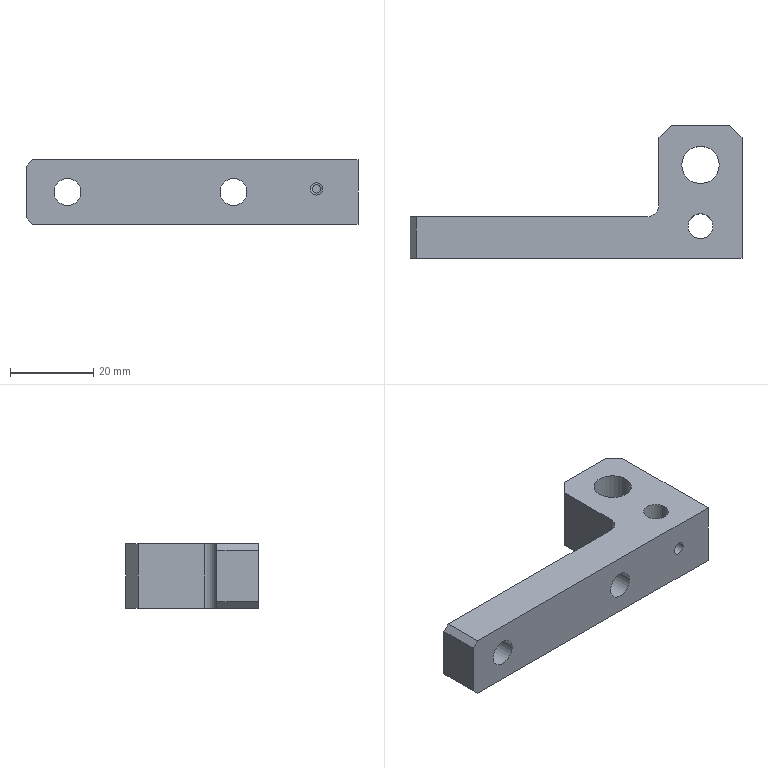NC program | NX | posted with a generic post | part box 80 x 32 x 15.5 mm
Lines 1 to 843 of 1848:
N10 G17 G21 G94 G90
(ADAPTIVE_MILLING , TOOL : D10-30-D10-75-3T-ROUGH)
N12 T01 M6
N14 G54
N16 G17 G0 G90 X-14.714 Y-27.953 B0. C0. S3000 M3
N18 G43 Z20. H1
N20 Z3.1
N22 G94 G1 X-14.735 Y-27.804 Z2.163 F1500.
N24 X-14.756 Y-27.656 Z1.792
N26 X-14.778 Y-27.507 Z1.52
N28 X-14.799 Y-27.359 Z1.3
N30 X-14.82 Y-27.21 Z1.116
N32 X-14.841 Y-27.062 Z0.958
N34 X-14.862 Y-26.913 Z0.82
N36 X-14.883 Y-26.765 Z0.7
N38 X-14.904 Y-26.616 Z0.595
N40 X-14.925 Y-26.467 Z0.502
N42 X-14.946 Y-26.319 Z0.421
N44 X-14.967 Y-26.17 Z0.35
N46 X-14.988 Y-26.022 Z0.29
N48 X-15.009 Y-25.873 Z0.238
N50 X-15.03 Y-25.725 Z0.195
N52 X-15.051 Y-25.576 Z0.161
N54 X-15.072 Y-25.428 Z0.134
N56 X-15.093 Y-25.279 Z0.115
N58 X-15.114 Y-25.131 Z0.104
N60 X-15.135 Y-24.982 Z0.1
N62 X-15.363 Y-23.368
N64 G3 X-16.363 Y-22.5 R1.01
N66 G2 X-19.774 Y-22.29 R16.737
N68 G3 X-25.917 Y-22.107 R71.98
N70 G1 X-30.851 Y-22.1
N72 G2 X-41.35 Y-22.08 R681.82
N74 X-45.596 Y-19.563 R5.775
N76 X-47.239 Y-15.194 R10.06
N78 X-47.576 Y-9.708 R40.211
N80 G1 X-47.6 Y-2.208
N82 X-47.597 Y15.46
N84 G2 X-45.145 Y20.047 R5.721
N86 X-40.851 Y21.717 R9.828
N88 X-35.168 Y22.076 R39.146
N90 G1 X-27.668 Y22.1
N92 X40.882 Y22.099
N94 G2 X45.469 Y19.73 R5.695
N96 X47.205 Y15.397 R9.72
N98 X47.575 Y9.765 R37.875
N100 G3 X47.629 Y6.228 R103.503
N102 G1 X47.728 Y5.055
N104 X47.904 Y4.474
N106 G2 X48. Y1.85 R17.179
N108 G3 X48.45 Y1.015 R1.001
N110 G1 X48.82 Y0.771
N112 X50.479 Y-0.322 Z0.2
N114 X50.822 Y-0.56 F15000.
N116 G2 X51.159 Y-1.309 R1.002
N118 G1 Y-16.392
N120 G2 X50.282 Y-20.805 R11.534
N122 G1 X49.642 Y-22.35
N124 G2 X48.185 Y-23.956 R3.345
N126 G1 X47.336 Y-24.376
N128 X46.477 Y-24.773
N130 G2 X43.308 Y-25.416 R8.24
N132 G1 X-15.817 Y-25.563
N134 G2 X-16.613 Y-25.173 R1.002
N136 G1 X-16.748 Y-24.997
N138 X-17.958 Y-23.423 Z0.1 F1500.
N140 X-18.252 Y-23.036
N142 X-18.556 Y-22.657
N144 G3 X-18.977 Y-22.403 R1.021
N146 X-22.436 Y-21.831 R12.422
N148 X-31.452 Y-21.701 R185.205
N150 G2 X-39.651 Y-21.68 R445.211
N152 X-45.227 Y-18.167 R7.162
N154 X-46.837 Y-13.315 R12.369
N156 X-47.177 Y-7.178 R49.965
N158 G1 X-47.199 Y0.522
N160 X-47.197 Y13.772
N162 G2 X-43.863 Y19.608 R7.09
N164 X-39.039 Y21.306 R11.953
N166 X-33.005 Y21.673 R45.882
N168 G1 X-25.305 Y21.699
N170 X39.193 Y21.698
N172 G2 X45.156 Y18.278 R7.123
N174 X46.818 Y13.441 R12.136
N176 X47.18 Y7.764 R49.503
N178 G3 X47.306 Y6.049 R15.738
N180 X47.62 Y5.412 R8.746
N182 G1 X47.736 Y5.029
N184 G3 X48.524 Y4.331 R1.009
N186 G1 X50.454 Y3.861 Z0.2
N188 X50.72 Y3.798 F15000.
N190 X50.983 Y3.721
N192 G2 X51.605 Y2.795 R1.001
N194 G1 Y-13.34
N196 G2 X51.071 Y-18.246 R22.814
N198 G1 X50.896 Y-19.053
N200 X50.704 Y-19.856
N202 G2 X47.108 Y-24.346 R7.33
N204 X46.142 Y-24.761 R7.288
N206 X44.228 Y-25.327 R15.44
N208 X41.944 Y-25.575 R11.567
N210 G1 X-17.413 Y-26.07
N212 G2 X-18.393 Y-25.303 R1.
N214 G1 X-18.473 Y-24.97
N216 X-18.937 Y-23.039 Z0.1 F1500.
N218 G3 X-19.508 Y-22.254 R1.059
N220 X-21.032 Y-21.765 R13.134
N222 X-25.727 Y-21.363 R28.488
N224 X-37.951 Y-21.289 R754.678
N226 G2 X-44.901 Y-16.95 R8.103
N228 X-46.45 Y-11.759 R14.331
N230 X-46.78 Y-4.971 R60.69
N232 G1 X-46.799 Y2.229
N234 X-46.783 Y12.579
N236 G2 X-42.478 Y19.387 R8.083
N238 X-37.238 Y20.954 R14.336
N240 X-30.45 Y21.28 R61.3
N242 G1 X-23.25 Y21.299
N244 X37.6 Y21.297
N246 G2 X44.907 Y16.935 R8.122
N248 X46.432 Y11.892 R14.201
N250 X46.81 Y7.334 R102.693
N252 G3 X47.059 Y6.399 R2.011
N254 X47.508 Y6.062 R1.012
N256 G1 X48.471 Y5.702
N258 X50.33 Y5.003 Z0.2
N260 G2 X50.929 Y4.165 R1.001 F15000.
N262 G1 X51.038 Y2.776
N264 X51.138 Y1.386
N266 G2 X51.198 Y-1.397 R42.642
N268 G1 X50.998 Y-17.535
N270 G2 X50.112 Y-21.491 R9.773
N272 X48.101 Y-23.985 R6.903
N274 X46.76 Y-24.887 R8.194
N276 X43.683 Y-25.648 R6.743
N278 G1 X-17.725 Y-25.965
N280 G2 X-18.686 Y-25.258 R1.
N282 G1 X-18.785 Y-24.934
N284 X-19.367 Y-23.035 Z0.1 F1500.
N286 X-19.521 Y-22.562
N288 G3 X-19.959 Y-22.095 R1.007
N290 X-22.533 Y-21.285 R6.797
N292 X-28.518 Y-20.935 R48.284
N294 G2 X-36.851 Y-20.878 R946.687
N296 X-44.518 Y-15.953 R8.819
N298 X-46.04 Y-10.591 R15.704
N300 X-46.381 Y-3.253 R67.006
N302 X-46.376 Y11.371 R824.313
N304 X-41.497 Y18.996 R8.797
N306 X-36.243 Y20.521 R15.472
N308 X-29.206 Y20.877 R62.007
N310 G1 X-22.556 Y20.898
N312 X36.044 Y20.897
N314 G2 X40.776 Y19.847 R9.724
N316 X44.932 Y15.065 R9.404
N318 X46.128 Y9.92 R18.692
N320 G3 X46.498 Y7.297 R19.933
N322 X46.7 Y6.835 R1.928
N324 G2 X47.37 Y5.88 R3.796
N326 G3 X47.958 Y5.395 R1.003
N328 G1 X48.481 Y5.234
N330 X50.379 Y4.649 Z0.2
N332 G2 X50.901 Y4.395 R1.246 F15000.
N334 X51.24 Y3.646 R1.002
N336 G1 Y-16.402
N338 G2 X50.362 Y-20.814 R11.534
N340 G1 X49.722 Y-22.36
N342 G2 X48.475 Y-23.837 R3.306
N344 G1 X48.264 Y-23.964
N346 X48.047 Y-24.08
N348 X47.306 Y-24.438
N350 X46.558 Y-24.785
N352 G2 X43.39 Y-25.434 R8.262
N354 G1 X-18.166 Y-25.729
N356 G2 X-19.127 Y-25.022 R1.
N358 G1 X-19.165 Y-24.897
N360 X-19.747 Y-22.998 Z0.1 F1500.
N362 X-19.848 Y-22.66
N364 X-19.961 Y-22.326
N366 G3 X-20.4 Y-21.859 R1.007
N368 X-23.33 Y-20.912 R7.518
N370 X-29.573 Y-20.539 R50.382
N372 G2 X-35.961 Y-20.462 R274.783
N374 X-44.066 Y-15.175 R9.369
N376 X-45.634 Y-9.52 R16.775
N378 X-45.981 Y-1.931 R71.604
N380 X-45.973 Y10.221 R586.173
N382 X-43.583 Y16.38 R9.462
N384 X-38.344 Y19.481 R11.217
N386 X-32.27 Y20.36 R26.687
N388 X-21.022 Y20.498 R255.072
N390 G1 X34.594
N392 G2 X38.925 Y19.873 R12.356
N394 X44.169 Y14.966 R9.478
N396 X45.61 Y9.987 R17.983
N398 G3 X46.186 Y7.447 R12.718
N400 G1 X46.387 Y7.162
N402 G3 X47.1 Y6.879 R1.003
N404 G1 X47.641 Y6.888
N406 X49.627 Y6.919 Z0.2
N408 G2 X50.703 Y6.005 R1.004 F15000.
N410 G1 X50.863 Y4.153
N412 X50.99 Y2.299
N414 X51.028 Y1.37
N416 X51.055 Y0.442
N418 X51.364 Y-16.831
N420 G2 X50.537 Y-20.562 R8.179
N422 G1 X50.288 Y-21.071
N424 X50.03 Y-21.576
N426 G2 X46.414 Y-24.768 R7.185
N428 X44.441 Y-25.299 R8.502
N430 X41.978 Y-25.475 R17.725
N432 G1 X-18.545 Y-25.526
N434 G2 X-19.493 Y-24.847 R1.001
N436 G1 X-20.158 Y-22.976 Z0.1 F1500.
N438 X-20.334 Y-22.47
N440 X-20.525 Y-21.97
N442 G3 X-20.779 Y-21.656 R1.063
N444 X-22.712 Y-20.797 R4.681
N446 X-27.729 Y-20.221 R26.336
N448 X-34.584 Y-20.082 R457.494
N450 G2 X-39.917 Y-18.597 R10.707
N452 X-44.138 Y-13.279 R10.563
N454 X-45.351 Y-7.32 R21.539
N456 X-45.593 Y1.724 R122.623
N458 X-45.559 Y9.373 R222.08
N460 X-43.559 Y15.194 R10.168
N462 X-38.192 Y18.849 R11.065
N464 X-32.399 Y19.884 R23.65
N466 X-23.553 Y20.093 R136.651
N468 G1 X-19.703 Y20.098
N470 X33.394 Y20.097
N472 G2 X37.65 Y19.605 R14.796
N474 X43.577 Y14.536 R9.791
N476 X45.047 Y10.239 R18.608
N478 G3 X45.719 Y7.923 R14.432
N480 X46.028 Y7.452 R1.701
N482 G2 X46.727 Y6.802 R3.41
N484 G3 X47.585 Y6.44 R1.001
N486 G1 X47.802 Y6.459
N488 X49.781 Y6.627 Z0.2
N490 G2 X50.401 Y6.58 R1.287 F15000.
N492 X51.043 Y5.646 R1.
N494 G1 Y-17.936
N496 G2 X50.402 Y-20.7 R6.428
N498 X48.791 Y-23.066 R8.698
N500 X47.097 Y-24.351 R7.72
N502 X44.507 Y-25.378 R9.704
N504 X42.88 Y-25.56 R7.773
N506 G1 X-19.777 Y-25.845
N508 G2 X-20.778 Y-24.759 R1.
N510 G1 X-20.753 Y-24.478
N512 X-20.582 Y-22.499 Z0.1 F1500.
N514 G3 X-20.934 Y-21.529 R1.045
N516 X-22.985 Y-20.51 R4.814
N518 X-27.996 Y-19.854 R24.391
N520 X-33.776 Y-19.684 R611.585
N522 G2 X-39.086 Y-18.255 R11.47
N524 X-43.596 Y-12.838 R10.785
N526 X-44.915 Y-6.75 R21.373
N528 X-45.187 Y1.644 R105.147
N530 X-45.145 Y8.593 R150.97
N532 X-43.224 Y14.396 R10.761
N534 X-37.757 Y18.316 R11.24
N536 X-31.581 Y19.47 R23.765
N538 X-22.436 Y19.693 R137.445
N540 G1 X-18.586 Y19.698
N542 X32.194 Y19.697
N544 G2 X36.561 Y19.274 R17.525
N546 X43.087 Y13.962 R10.184
N548 X44.682 Y9.777 R24.402
N550 G3 X45.475 Y7.906 R7.211
N552 G1 X45.696 Y7.705
N554 G3 X46.557 Y7.598 R1.002
N556 G1 X46.808 Y7.683
N558 X48.689 Y8.319 Z0.2
N560 G2 X49.171 Y8.436 R1.518 F15000.
N562 X50.164 Y7.705 R1.
N564 G1 X50.622 Y6.031
N566 G2 X50.941 Y4.08 R13.684
N568 G1 X51.268 Y0.429
N570 X51.578 Y-3.223
N572 G2 X51.364 Y-14.453 R62.802
N574 G1 X50.826 Y-19.388
N576 G2 X49.721 Y-22.298 R6.117
N578 X48.484 Y-23.515 R5.386
N580 G1 X47.817 Y-23.988
N582 X47.141 Y-24.451
N584 G2 X42.969 Y-25.655 R7.799
N586 G1 X-20.086 Y-25.592
N588 G2 X-21.082 Y-24.507 R1.
N590 G1 X-21.068 Y-24.343
N592 X-20.9 Y-22.364 Z0.1 F1500.
N594 G3 X-20.896 Y-21.858 R1.79
N596 X-21.243 Y-21.276 R1.006
N598 X-23.549 Y-20.135 R5.314
N600 X-28.561 Y-19.471 R25.379
N602 G2 X-33.533 Y-19.255 R236.762
N604 X-39.442 Y-17.168 R11.236
N606 X-43.388 Y-11.566 R11.676
N608 X-44.562 Y-5.242 R24.608
N610 X-44.794 Y4.904 R151.502
N612 X-44.553 Y9.391 R26.845
N614 X-38.661 Y17.215 R10.493
N616 X-32.663 Y18.872 R18.654
N618 X-24.478 Y19.274 R74.416
N620 G1 X-17.278 Y19.297
N622 X31.044 Y19.296
N624 G2 X35.617 Y18.907 R20.31
N626 X42.471 Y13.68 R10.564
N628 X44.188 Y9.842 R28.498
N630 G3 X45.156 Y8.035 R6.211
N632 X45.779 Y7.656 R2.99
N634 G1 X46.049 Y7.434
N636 G3 X47.052 Y7.277 R1.001
N638 G1 X48.847 Y8.126 Z0.2
N640 X49.037 Y8.215 F15000.
N642 X49.231 Y8.296
N644 G2 X50.518 Y7.434 R1.
N646 G1 X50.812 Y4.348
N648 X51.07 Y1.259
N650 X51.171 Y-0.287
N652 X51.257 Y-1.835
N654 X51.56 Y-8.036
N656 G2 X51.183 Y-16.678 R46.836
N658 G1 X50.845 Y-19.138
N660 G2 X47.709 Y-24.114 R7.078
N662 X46.137 Y-24.88 R7.94
N664 X42.754 Y-25.485 R9.772
N666 G1 X-19.527
N668 G2 X-20.515 Y-25.308 R3.366
N670 X-21.146 Y-24.436 R1.001
N672 G1 X-21.155 Y-24.295
N674 X-21.27 Y-22.313 Z0.1 F1500.
N676 X-21.291 Y-21.899
N678 X-21.327 Y-21.486
N680 G3 X-21.536 Y-21.034 R1.02
N682 X-23.105 Y-20.065 R3.781
N684 X-27.529 Y-19.203 R17.384
N686 X-32.711 Y-18.879 R747.688
N688 G2 X-38.324 Y-17.094 R12.112
N690 X-42.791 Y-11.371 R11.636
N692 X-44.09 Y-5.226 R22.987
N694 X-44.387 Y3.866 R110.396
N696 X-44.148 Y8.605 R29.152
N698 X-37.994 Y16.799 R10.818
N700 X-31.943 Y18.456 R19.235
N702 X-23.958 Y18.868 R72.763
N704 G1 X-15.108 Y18.897
N706 X29.992 Y18.896
N708 G2 X34.719 Y18.534 R22.942
N710 X41.806 Y13.513 R10.976
N712 X43.741 Y9.797 R34.512
N714 G3 X44.712 Y8.257 R6.177
N716 X45.37 Y7.875 R5.475
N718 X46.062 Y7.781 R1.005
N720 G1 X46.716 Y7.929
N722 X48.653 Y8.366 Z0.2
N724 G2 X49.838 Y7.875 R1.018 F15000.
N726 G1 X50.344 Y6.923
N728 X50.835 Y5.964
N730 G2 X51.491 Y2.974 R7.15
N732 G1 Y-15.114
N734 G2 X50.706 Y-19.952 R15.305
N736 G1 X50.465 Y-20.685
N738 X50.208 Y-21.413
N740 G2 X48.991 Y-23.133 R4.646
N742 X46.488 Y-24.669 R8.641
N744 X42.156 Y-25.524 R11.366
N746 G1 X-18.513 Y-25.391
N748 G2 X-20.443 Y-25.273 R19.912
N750 X-21.353 Y-24.285 R1.
N752 G1 X-21.354 Y-24.185
N754 X-21.368 Y-22.199 Z0.1 F1500.
N756 Y-21.823
N758 X-21.383 Y-21.448
N760 G3 X-21.6 Y-20.957 R1.014
N762 X-23.279 Y-19.799 R3.75
N764 X-27.648 Y-18.86 R16.456
N766 G2 X-32.453 Y-18.459 R331.016
N768 X-38.453 Y-16.169 R12.057
N770 X-42.483 Y-10.425 R12.3
N772 X-43.731 Y-3.911 R25.337
N774 X-43.908 Y6.332 R91.067
N776 X-42.178 Y12.167 R12.335
N778 X-36.453 Y16.777 R11.742
N780 X-30.074 Y18.172 R22.995
N782 X-21.182 Y18.484 R105.943
N784 G1 X-15.132 Y18.497
N786 X28.994 Y18.496
N788 G2 X33.825 Y18.162 R25.814
N790 X41.234 Y13.226 R11.502
N792 X43.295 Y9.764 R46.583
N794 G3 X44.401 Y8.324 R5.147
N796 X44.959 Y8.095 R3.127
N798 X45.997 Y8.153 R1.001
N800 G1 X46.753 Y8.795 Z0.15
N802 X47.501 Y9.448 Z0.2
N804 X47.814 Y9.706 F15000.
N806 G2 X49.275 Y9.252 R1.
N808 G1 X49.828 Y7.946
N810 X50.365 Y6.634
N812 G2 X51.08 Y2.638 R11.526
N814 G1 Y-17.377
N816 G2 X50.245 Y-20.945 R8.234
N818 X47.7 Y-24.037 R8.218
N820 X45.037 Y-25.198 R7.143
N822 X43.408 Y-25.39 R8.463
N824 X27.901 Y-25.602 R952.924
N826 G1 X-16.916 Y-25.805
N828 G2 X-19.414 Y-25.426 R8.19
N830 G1 X-20.634 Y-25.041
N832 G2 X-21.326 Y-24.204 R1.001
N834 G1 X-21.489 Y-22.224 Z0.1 F1500.
N836 X-21.567 Y-21.277
N838 G3 X-21.79 Y-20.725 R1.009
N840 X-23.62 Y-19.455 R4.102
N842 X-27.899 Y-18.503 R16.744
N844 G2 X-32.357 Y-18.012 R95.294
N846 X-38.865 Y-14.917 R11.936
N848 X-42.31 Y-9.054 R13.4
N850 X-43.39 Y-2.254 R29.777
N852 X-43.484 Y5.741 R70.346
N854 X-41.671 Y11.706 R12.569
N856 X-35.842 Y16.352 R12.01
N858 X-29.463 Y17.754 R23.409
N860 X-20.022 Y18.085 R108.737
N862 G1 X-13.422 Y18.097
N864 X27.944 Y18.096
N866 G2 X32.879 Y17.8 R29.782
N868 X40.639 Y13.003 R12.088
N870 X42.891 Y9.671 R70.619
N872 G3 X44.018 Y8.419 R4.824
N874 X44.67 Y8.193 R6.088
N876 X45.472 Y8.291 R1.002
N878 G1 X45.76 Y8.463
N880 X47.466 Y9.48 Z0.2
N882 G2 X47.945 Y9.716 R1.786 F15000.
N884 X48.986 Y9.35 R1.001
N886 G1 X49.539 Y8.603
N888 G2 X49.977 Y7.789 R5.276
N890 X50.496 Y6.446 R12.486
N892 X50.787 Y4.836 R7.473
N894 X51.502 Y-6.926 R544.363
N896 G1 X51.773 Y-12.507
N898 G2 X51.324 Y-17.403 R17.642
N900 X50.653 Y-19.783 R19.367
N902 X49.925 Y-21.486 R16.68
N904 G1 X49.596 Y-22.152
N906 X49.254 Y-22.812
N908 G2 X47.588 Y-24.203 R3.415
N910 G1 X46.8 Y-24.516
N912 X46.007 Y-24.82
N914 G2 X42.856 Y-25.409 R10.722
N916 X35.414 Y-25.572 R219.894
N918 G1 X-14.892 Y-25.77
N920 G2 X-19.629 Y-25.37 R27.069
N922 G1 X-21.98 Y-24.961
N924 G2 X-22.726 Y-23.578 R1.
N926 G1 X-22.637 Y-23.372
N928 X-21.847 Y-21.55 Z0.1 F1500.
N930 G3 X-21.98 Y-20.493 R1.002
N932 X-23.81 Y-19.167 R4.163
N934 X-28.123 Y-18.143 R16.733
N936 G2 X-32.515 Y-17.5 R48.24
N938 X-41.146 Y-10.451 R11.983
N940 X-42.773 Y-3.979 R21.871
N942 X-43.057 Y5.157 R57.101
N944 X-41.195 Y11.209 R12.776
N946 X-35.417 Y15.859 R12.175
N948 X-28.953 Y17.328 R23.307
N950 X-20.013 Y17.679 R99.589
N952 G1 X-12.313 Y17.696
N954 X26.994
N956 G2 X32.13 Y17.405 R32.538
N958 X40.045 Y12.797 R12.721
N960 X42.478 Y9.6 R124.49
N962 G3 X43.634 Y8.493 R4.133
N964 G1 X43.871 Y8.417
N966 G3 X44.4 Y8.471 R1.015
N968 G1 X45.462 Y8.884
N970 X47.313 Y9.604 Z0.2
N972 G2 X48.187 Y9.573 R1.007 F15000.
N974 G1 X48.551 Y9.382
N976 X48.909 Y9.181
N978 G2 X49.593 Y8.455 R2.149
N980 X50.27 Y7.184 R13.138
N982 X50.858 Y5.137 R8.475
N984 X51.033 Y3.167 R13.068
N986 G1 X51.252 Y-16.07
N988 G2 X50.737 Y-19.715 R12.193
N990 X50.28 Y-21.079 R12.464
N992 X49.475 Y-22.504 R7.459
N994 G1 X48.962 Y-23.202
N996 G2 X47.706 Y-24.174 R3.97
N998 G1 X47.426 Y-24.304
N1000 X47.14 Y-24.42
N1002 X46.341 Y-24.707
N1004 X45.54 Y-24.985
N1006 G2 X42.37 Y-25.474 R10.783
N1008 G1 X-15.951 Y-25.695
N1010 G2 X-20.107 Y-25.224 R17.998
N1012 G1 X-22.158 Y-24.745
N1014 G2 X-22.88 Y-23.458 R1.
N1016 G1 X-22.806 Y-23.232
N1018 X-22.184 Y-21.345 Z0.1 F1500.
N1020 X-22.057 Y-20.93
N1022 G3 X-22.158 Y-20.277 R1.006
N1024 X-23.461 Y-19.138 R3.179
N1026 X-27.214 Y-17.961 R12.57
N1028 G2 X-31.56 Y-17.232 R128.383
N1030 X-38.104 Y-13.796 R12.68
N1032 X-41.535 Y-7.652 R14.264
N1034 X-42.58 Y-0.846 R31.757
N1036 X-42.544 Y5.396 R36.432
N1038 X-39.236 Y12.572 R11.918
N1040 X-33.208 Y16.006 R13.933
N1042 X-26.354 Y17.078 R31.236
N1044 X-16.258 Y17.291 R179.235
N1046 G1 X-12.408 Y17.296
N1048 X26.044 Y17.295
N1050 G2 X31.331 Y17.021 R36.056
N1052 X39.372 Y12.686 R13.362
N1054 X41.996 Y9.602 R152.403
N1056 G3 X43.291 Y8.51 R4.48
N1058 X43.977 Y8.403 R2.97
N1060 G1 X44.216 Y8.331
N1062 G3 X45.019 Y8.429 R1.002
N1064 G1 X45.462 Y8.693
N1066 X47.168 Y9.71 Z0.2
N1068 G2 X48.532 Y9.487 R1.004 F15000.
N1070 G1 X49.205 Y8.604
N1072 X49.864 Y7.709
N1074 G2 X50.84 Y4.658 R5.858
N1076 G1 X51.423 Y-13.327
N1078 G2 X51.012 Y-18.241 R21.35
N1080 G1 X50.852 Y-19.051
N1082 X50.674 Y-19.856
N1084 G2 X46.786 Y-24.513 R7.226
N1086 G1 X46.176 Y-24.761
N1088 X45.554 Y-24.977
N1090 G2 X41.941 Y-25.601 R11.373
N1092 G1 X-15.353 Y-26.118
N1094 G2 X-19.961 Y-25.398 R14.286
N1096 G1 X-22.205 Y-24.657
N1098 G2 X-22.852 Y-23.427 R1.
N1100 G1 X-22.797 Y-23.239
N1102 X-22.242 Y-21.332 Z0.1 F1500.
N1104 X-22.161 Y-21.062
N1106 X-22.095 Y-20.788
N1108 G3 X-22.205 Y-20.188 R1.008
N1110 X-23.553 Y-18.893 R3.189
N1112 X-27.192 Y-17.651 R12.329
N1114 G2 X-31.493 Y-16.777 R85.932
N1116 X-38.639 Y-12.184 R12.736
N1118 X-41.419 Y-5.914 R16.156
N1120 X-42.146 Y4.426 R37.118
N1122 X-39.59 Y11.159 R12.447
N1124 X-33.674 Y15.243 R13.13
N1126 X-26.974 Y16.576 R26.481
N1128 X-16.831 Y16.886 R129.626
N1130 G1 X-10.231 Y16.896
N1132 X25.094 Y16.895
N1134 G2 X30.682 Y16.617 R38.826
N1136 X38.848 Y12.421 R14.152
N1138 X41.542 Y9.553 R554.574
N1140 G3 X42.877 Y8.54 R4.702
N1142 X43.569 Y8.444 R5.472
N1144 X44.528 Y8.93 R1.001
N1146 X44.612 Y9.781 Z0.144 R1.045
N1148 G1 X44.332 Y10.85 Z0.2
N1150 X43.936 Y12.365 F15000.
N1152 G3 X43.569 Y12.912 R1.007
N1154 G1 X39.101 Y16.263
N1156 G3 X35.921 Y18.16 R17.61
N1158 X33.978 Y18.968 R17.349
N1160 X30.585 Y19.609 R12.289
N1162 X22.529 Y19.89 R269.637
N1164 G1 X20.669 Y19.914
N1166 X-19.67 Y20.246
N1168 G3 X-28.298 Y19.563 R49.697
N1170 G1 X-29.827 Y19.309
N1172 X-31.355 Y19.041
N1174 G3 X-37.676 Y16.617 R19.744
N1176 X-40.237 Y14.882 R21.016
N1178 X-41.948 Y13.111 R9.713
N1180 G1 X-42.928 Y11.78
N1182 G3 X-44.396 Y8.574 R10.905
N1184 X-44.739 Y7.005 R17.751
N1186 X-45.221 Y2.702 R28.858
N1188 X-45.068 Y-2.242 R29.686
N1190 G1 X-44.922 Y-3.514
N1192 X-44.766 Y-4.784
N1194 G3 X-43.184 Y-10.57 R24.032
N1196 X-40.1 Y-15.123 R14.552
N1198 G1 X-39.293 Y-15.933
N1200 X-38.476 Y-16.734
N1202 G3 X-36.376 Y-18.166 R9.211
N1204 X-34.551 Y-18.928 R13.2
N1206 X-30.396 Y-20.166 R56.304
N1208 G1 X-26.56 Y-21.141
N1210 X-24.43 Y-21.334
N1212 X-23.223 Y-21.436 Z0.139 F1500.
N1214 G3 X-22.519 Y-21.166 Z0.1 R1.
N1216 X-22.323 Y-19.968 R1.
N1218 X-23.776 Y-18.566 R3.419
N1220 X-27.257 Y-17.319 R12.904
N1222 G2 X-31.668 Y-16.237 R54.867
N1224 X-40.009 Y-8.517 R13.072
N1226 X-41.581 Y-1.767 R24.151
N1228 X-41.591 Y4.767 R27.221
N1230 X-34.68 Y14.164 R12.047
N1232 X-28.2 Y15.964 R21.282
N1234 X-19.569 Y16.455 R75.11
N1236 X-9.669 Y16.495 R706.736
N1238 G1 X24.144
N1240 G2 X29.933 Y16.229 R43.047
N1242 X38.36 Y12.135 R15.041
N1244 G3 X41.15 Y9.436 R309.311
N1246 X42.534 Y8.528 R4.073
N1248 G1 X43.1 Y8.49
N1250 G3 X44.165 Y9.23 R1.
N1252 X43.939 Y10.164 Z0.15 R1.043
N1254 G1 X43.348 Y10.952 Z0.2
N1256 X42.036 Y12.699 F15000.
N1258 X41.944 Y12.806
N1260 X41.068 Y13.684
N1262 X40.183 Y14.552
N1264 G3 X36.389 Y17.271 R17.722
N1266 X32.688 Y18.672 R17.552
N1268 X28.667 Y19.309 R23.068
N1270 G1 X27.927 Y19.351
N1272 X27.186 Y19.375
N1274 X-15.012 Y20.009
N1276 G3 X-26.13 Y19.332 R73.571
N1278 G1 X-28.281 Y19.04
N1280 X-30.43 Y18.731
N1282 G3 X-37.432 Y16.059 R18.893
N1284 X-40.661 Y13.699 R28.808
N1286 X-42.282 Y11.747 R8.431
N1288 X-43.156 Y9.977 R11.018
N1290 G1 X-43.603 Y8.827
N1292 X-44.033 Y7.672
N1294 G3 X-44.937 Y2.256 R16.632
N1296 X-44.32 Y-4.519 R38.652
N1298 X-42.79 Y-9.708 R23.219
N1300 X-40.852 Y-13.182 R16.477
N1302 X-39.473 Y-14.956 R22.606
N1304 X-37.276 Y-16.941 R12.041
N1306 X-34.652 Y-18.316 R13.043
N1308 X-30.562 Y-19.749 R52.554
N1310 G1 X-26.757 Y-20.904
N1312 X-26.552 Y-20.943
N1314 X-24.546 Y-21.116
N1316 X-23.339 Y-21.216 Z0.139 F1500.
N1318 G3 X-22.635 Y-20.945 Z0.1 R1.
N1320 X-22.441 Y-19.747 R1.
N1322 X-23.876 Y-18.304 R3.48
N1324 X-27.356 Y-16.97 R13.39
N1326 G2 X-31.788 Y-15.683 R41.644
N1328 X-39.616 Y-7.934 R13.436
N1330 X-41.216 Y-0.581 R24.877
N1332 X-40.887 Y5.535 R19.844
N1334 X-34.454 Y13.584 R12.05
N1336 X-27.91 Y15.512 R20.777
N1338 X-19.832 Y16.038 R67.518
N1340 X-8.632 Y16.095 R719.502
N1342 G1 X23.318
N1344 G2 X29.307 Y15.827 R45.585
N1346 X37.701 Y12.007 R15.84
N1348 G3 X40.762 Y9.311 R181.567
N1350 X42.11 Y8.52 R4.038
N1352 G1 X42.758 Y8.5
N1354 G3 X43.722 Y9.232 R1.
N1356 X43.522 Y10.152 Z0.149 R1.04
N1358 G1 X42.941 Y10.975 Z0.2
N1360 X41.769 Y12.632 F15000.
N1362 X41.689 Y12.728
N1364 X41.602 Y12.816
N1366 G3 X39.379 Y14.656 R52.718
N1368 G1 X38.585 Y15.245
N1370 X37.779 Y15.819
N1372 G3 X34.968 Y17.275 R14.162
N1374 X31.009 Y18.475 R22.809
N1376 X28.634 Y18.823 R28.225
N1378 X24.681 Y19.08 R46.073
N1380 G1 X-7.585 Y19.773
N1382 G3 X-22.436 Y19.148 R117.146
N1384 G1 X-25.257 Y18.853
N1386 X-28.075 Y18.542
N1388 G3 X-32.819 Y17.492 R29.162
N1390 X-36.674 Y15.91 R19.755
N1392 X-39.236 Y13.962 R11.495
N1394 G1 X-40.066 Y13.126
N1396 X-40.884 Y12.278
N1398 G3 X-43.097 Y8.454 R10.967
N1400 X-43.911 Y5.481 R20.179
N1402 G1 X-44.011 Y4.872
N1404 X-44.093 Y4.26
N1406 X-44.235 Y3.028
N1408 X-44.363 Y1.795
N1410 G3 X-44.217 Y-2.512 R18.897
N1412 X-42.898 Y-7.917 R30.47
N1414 X-41.033 Y-11.807 R20.14
N1416 X-39.792 Y-13.629 R16.954
N1418 X-37.398 Y-15.96 R14.284
N1420 X-35.045 Y-17.483 R16.826
N1422 X-31.043 Y-19.249 R23.877
N1424 G1 X-26.898 Y-20.639
N1426 X-26.664 Y-20.688
N1428 X-24.685 Y-20.854
N1430 X-23.478 Y-20.951 Z0.139 F1500.
N1432 G3 X-22.775 Y-20.678 Z0.1 R1.
N1434 X-22.582 Y-19.483 R1.
N1436 X-23.921 Y-18.072 R3.4
N1438 X-27.231 Y-16.677 R13.192
N1440 G2 X-31.623 Y-15.224 R41.027
N1442 X-39.269 Y-7.246 R13.864
N1444 X-40.687 Y3.515 R23.871
N1446 X-33.892 Y13.177 R12.168
N1448 X-27.494 Y15.078 R20.862
N1450 X-19.169 Y15.636 R66.744
N1452 X-7.619 Y15.695 R728.649
N1454 G1 X22.431 Y15.694
N1456 G2 X28.572 Y15.441 R50.05
N1458 X37.124 Y11.801 R16.774
N1460 G3 X40.203 Y9.304 R243.468
N1462 X41.6 Y8.519 R4.57
N1464 G1 X42.299 Y8.5
N1466 G3 X43.261 Y9.228 R1.
N1468 X43.066 Y10.148 Z0.149 R1.04
N1470 G1 X42.489 Y10.975 Z0.2
N1472 X41.897 Y11.826 F15000.
N1474 X41.297 Y12.672
N1476 X41.142 Y12.816
N1478 X40.15 Y13.56
N1480 X39.153 Y14.297
N1482 G3 X36.506 Y15.897 R21.885
N1484 G1 X35.681 Y16.319
N1486 X34.851 Y16.731
N1488 G3 X30.743 Y18.042 R17.916
N1490 X27.677 Y18.442 R25.331
N1492 X22.727 Y18.72 R85.062
N1494 G1 X5.359 Y19.182
N1496 G3 X-16.96 Y18.847 R268.84
N1498 G1 X-26.254 Y18.321
N1500 G3 X-36.229 Y15.291 R22.297
N1502 G1 X-37.28 Y14.637
N1504 X-38.32 Y13.963
N1506 X-38.699 Y13.695
N1508 X-39.068 Y13.413
N1510 G3 X-39.717 Y12.754 R5.199
N1512 X-41.822 Y9.698 R18.013
N1514 X-43.275 Y6.298 R15.742
N1516 X-43.818 Y4.108 R17.151
N1518 X-43.978 Y0.845 R13.844
N1520 X-42.928 Y-5.87 R34.198
N1522 X-42.208 Y-8.255 R22.761
N1524 X-40.673 Y-11.421 R19.577
N1526 X-35.501 Y-16.596 R14.033
N1528 X-32.186 Y-18.269 R34.293
N1530 G1 X-26.936 Y-20.568
N1532 G3 X-26.551 Y-20.652 R1.07
N1534 G1 X-24.779 Y-20.682
N1536 X-23.527 Y-20.699 Z0.137 F1500.
N1538 G3 X-22.871 Y-20.41 Z0.1 R1.001
N1540 X-22.62 Y-19.412 R1.001
N1542 X-23.69 Y-18.035 R2.812
N1544 X-26.723 Y-16.522 R11.04
N1546 G2 X-31.007 Y-14.97 R61.821
N1548 X-38.939 Y-6.524 R14.357
N1550 X-40.188 Y3.112 R21.576
N1552 X-33.528 Y12.67 R12.161
N1554 X-26.954 Y14.663 R20.807
N1556 X-18.779 Y15.229 R65.677
N1558 X-7.029 Y15.295 R723.505
N1560 G1 X21.571 Y15.294
N1562 G2 X27.962 Y15.041 R53.811
N1564 X36.752 Y11.444 R17.926
N1566 G3 X39.952 Y9.066 R78.782
N1568 X41.164 Y8.502 R3.193
N1570 G1 X41.752 Y8.5
N1572 G3 X42.712 Y9.219 R1.
N1574 X42.528 Y10.138 Z0.149 R1.04
N1576 G1 X41.959 Y10.975 Z0.2
N1578 X40.909 Y12.52 F15000.
N1580 G3 X40.596 Y12.816 R1.047
N1582 G1 X38.697 Y13.959
N1584 X36.789 Y15.088
N1586 G3 X28.131 Y17.931 R23.429
N1588 X23.19 Y18.315 R61.143
N1590 G1 X15.747 Y18.588
N1592 G3 X-4.098 Y18.659 R300.237
N1594 G1 X-23.949 Y18.073
N1596 G3 X-30.908 Y16.944 R26.494
N1598 X-34.606 Y15.484 R28.239
N1600 X-37.278 Y13.794 R14.24
N1602 X-39.632 Y11.781 R35.062
N1604 X-41.406 Y9.428 R9.003
N1606 X-42.193 Y7.615 R12.337
N1608 X-42.929 Y4.982 R17.49
N1610 X-43.136 Y3.409 R15.6
N1612 G1 X-43.232 Y2.174
N1614 X-43.315 Y0.939
N1616 G3 X-42.852 Y-4.049 R18.594
N1618 X-41.555 Y-8.08 R23.654
N1620 G1 X-41.091 Y-9.181
N1622 X-40.612 Y-10.275
N1624 G3 X-38.182 Y-13.708 R12.724
N1626 X-36.044 Y-15.528 R15.533
N1628 X-32.586 Y-17.619 R25.381
N1630 G1 X-26.979 Y-20.425
N1632 G3 X-26.541 Y-20.531 R1.039
N1634 G1 X-24.849 Y-20.547
N1636 X-24.201 Y-20.556 Z0.167 F1500.
N1638 X-23.553 Y-20.553 Z0.135
N1640 G3 X-22.933 Y-20.285 Z0.1 R1.001
N1642 X-22.663 Y-19.268 R1.001
N1644 X-23.721 Y-17.811 R2.893
N1646 X-26.821 Y-16.161 R11.575
N1648 G2 X-31.205 Y-14.351 R46.908
N1650 X-38.575 Y-5.892 R14.782
N1652 X-39.649 Y2.915 R19.364
N1654 X-33.235 Y12.125 R12.097
N1656 X-26.735 Y14.199 R20.293
N1658 X-18.814 Y14.811 R60.252
N1660 X-6.465 Y14.894 R612.413
N1662 G1 X21.335 Y14.893
N1664 G2 X27.575 Y14.615 R50.282
N1666 X36.28 Y11.17 R19.063
N1668 G3 X39.502 Y8.958 R66.329
N1670 X40.608 Y8.5 R2.775
N1672 G1 X41.208
N1674 G3 X42.166 Y9.214 R1.
N1676 X41.987 Y10.133 Z0.149 R1.04
N1678 G1 X41.422 Y10.975 Z0.2
N1680 X40.404 Y12.494 F15000.
N1682 G3 X40.051 Y12.816 R1.024
N1684 G1 X38.419 Y13.704